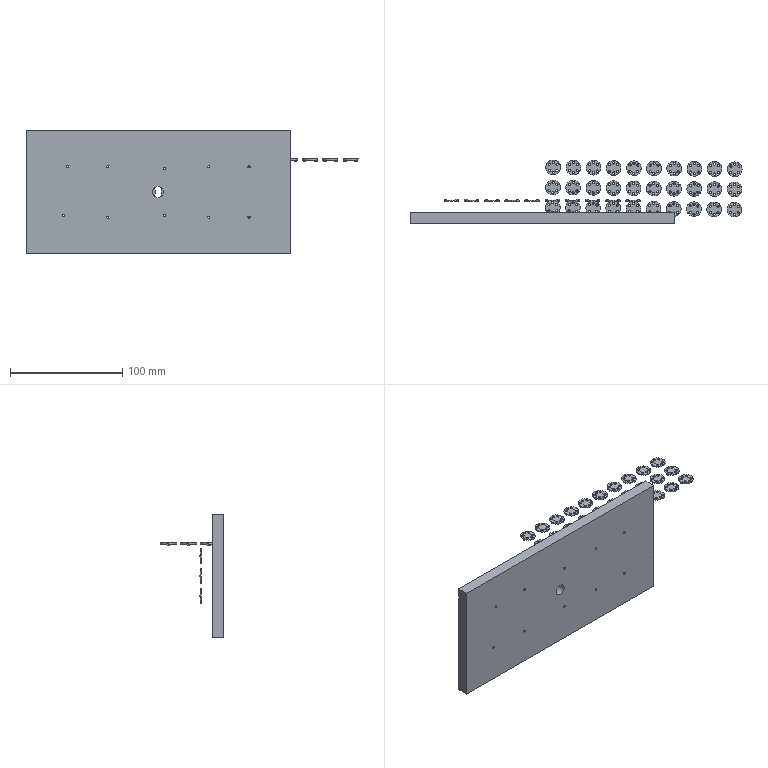NC program | NX | posted with a generic post | part box 296.27 x 56.878 x 110 mm
Lines 1 to 954 of 20851:
N10 G17 G21 G94 G90
(CAVITY_MILL_2 , TOOL : D3.R0)
N12 T03 M6
N14 G53
N16 G17 G0 G90 X-4.4 Y0. B0. C0. S4000 M3
N18 G43 Z10.1 H3
N20 G94 G1 Z-0.15 F5000.
N22 X-2.15 F2000.
N24 Y27.5
N26 G2 X-2. Y27.65 R0.15
N28 G1 X183.
N30 G2 X183.15 Y27.5 R0.15
N32 G1 Y-27.5
N34 G2 X183. Y-27.65 R0.15
N36 G1 X174.449
N38 G2 X168.332 Y-27.65 R8.4
N40 G1 X155.912
N42 G2 X150.871 Y-27.65 R8.4
N44 G1 X137.203
N46 G2 X133.582 Y-27.65 R8.4
N48 G1 X117.756
N50 G2 X117.031 Y-27.65 R8.4
N52 G1 X-2.
N54 G2 X-2.15 Y-27.5 R0.15
N56 G1 Y0.
N58 X-0.65
N60 Y26.15
N62 X8.318
N64 G3 X2.203 Y21.507 R8.4
N66 G1 X0.85 Y22.155
N68 Y24.65
N70 X2.557
N72 G3 X0.85 Y22.155 R9.9
N74 G1 X2.203 Y21.507
N76 G3 X11.239 Y26.15 R-8.4
N78 G1 X11.187 Y25.855
N80 G2 X17.755 Y16.47 R8.1
N82 X11.187 Y25.855 R-8.1
N84 G1 X11.239 Y26.15
N86 X23.077
N88 Y24.65
N90 G3 X19.558 Y19.419 R8.4
N92 X17. Y24.65 R9.9
N94 G1 X19.804
N96 Y23.3
N98 X19.71 Y23.163
N100 X19.636 Y23.3
N102 X19.804
N104 Y24.65
N106 X23.077
N108 Y26.15
N110 X181.65
N112 Y-26.15
N114 X176.92
N116 G3 X178.823 Y-23.741 R8.4
N118 G1 X180.15 Y-24.439
N120 Y-24.65
N122 X180.036
N124 G3 X180.15 Y-24.439 R9.9
N126 G1 X178.823 Y-23.741
N128 G3 X165.861 Y-26.15 R-8.4
N130 G1 X166.058 Y-25.924
N132 G2 X165.293 Y-14.495 R8.1
N134 X166.058 Y-25.924 R-8.1
N136 G1 X165.861 Y-26.15
N138 X158.696
N140 G3 X160.99 Y-23.217 R8.4
N142 G1 X162.347 Y-23.856
N144 G3 X162.745 Y-24.65 R9.9
N146 G1 X161.928
N148 G3 X162.347 Y-23.856 R9.9
N150 G1 X160.99 Y-23.217
N152 G3 X148.086 Y-26.15 R-8.4
N154 G1 X148.276 Y-25.917
N156 G2 X147.111 Y-14.522 R8.1
N158 X148.276 Y-25.917 R-8.1
N160 G1 X148.086 Y-26.15
N162 X140.455
N164 G3 X142.991 Y-23.027 R8.4
N166 G1 X144.348 Y-23.666
N168 G3 X144.854 Y-24.65 R9.9
N170 G1 X143.815
N172 G3 X144.348 Y-23.666 R9.9
N174 G1 X142.991 Y-23.027
N176 G3 X130.329 Y-26.15 R-8.4
N178 G1 X130.51 Y-25.911
N180 G2 X128.929 Y-14.565 R8.1
N182 X130.51 Y-25.911 R-8.1
N184 G1 X130.329 Y-26.15
N186 X122.195
N188 G3 X124.992 Y-22.837 R8.4
N190 G1 X126.349 Y-23.477
N192 G3 X126.881 Y-24.505 R9.9
N194 G1 X126.97 Y-24.65
N196 X125.696
N198 G3 X126.349 Y-23.477 R9.9
N200 G1 X124.992 Y-22.837
N202 G3 X112.591 Y-26.15 R-8.4
N204 G1 X112.763 Y-25.904
N206 G2 X110.747 Y-14.627 R8.1
N208 X112.763 Y-25.904 R-8.1
N210 G1 X112.591 Y-26.15
N212 X103.912
N214 G3 X106.993 Y-22.648 R8.4
N216 G1 X108.35 Y-23.287
N218 G3 X109.024 Y-24.547 R9.9
N220 G1 X109.091 Y-24.65
N222 X107.571
N224 G3 X108.35 Y-23.287 R9.9
N226 G1 X106.993 Y-22.648
N228 G3 X94.877 Y-26.15 R-8.4
N230 G1 X95.038 Y-25.897
N232 G2 X92.565 Y-14.712 R8.1
N234 X95.038 Y-25.897 R-8.1
N236 G1 X94.877 Y-26.15
N238 X85.601
N240 G3 X88.994 Y-22.458 R8.4
N242 G1 X90.351 Y-23.097
N244 G3 X91.218 Y-24.65 R9.9
N246 G1 X89.439
N248 G3 X90.351 Y-23.097 R9.9
N250 G1 X88.994 Y-22.458
N252 G3 X77.19 Y-26.15 R-8.4
N254 G1 X77.34 Y-25.89
N256 G2 X74.384 Y-14.823 R8.1
N258 X77.34 Y-25.89 R-8.1
N260 G1 X77.19 Y-26.15
N262 X67.255
N264 G3 X70.995 Y-22.269 R8.4
N266 G1 X72.352 Y-22.908
N268 G3 X73.352 Y-24.65 R9.9
N270 G1 X71.3
N272 G3 X72.352 Y-22.908 R9.9
N274 G1 X70.995 Y-22.269
N276 G3 X59.537 Y-26.15 R-8.4
N278 G1 X59.675 Y-25.884
N280 G2 X56.202 Y-14.968 R8.1
N282 X59.675 Y-25.884 R-8.1
N284 G1 X59.537 Y-26.15
N286 X48.865
N288 G3 X52.996 Y-22.079 R8.4
N290 G1 X54.353 Y-22.718
N292 G3 X55.492 Y-24.65 R9.9
N294 G1 X53.155
N296 G3 X54.353 Y-22.718 R9.9
N298 G1 X52.996 Y-22.079
N300 G3 X41.929 Y-26.15 R-8.4
N302 G1 X42.053 Y-25.877
N304 G2 X38.02 Y-15.155 R8.1
N306 X42.053 Y-25.877 R-8.1
N308 G1 X41.929 Y-26.15
N310 X30.413
N312 G3 X34.997 Y-21.889 R8.4
N314 G1 X36.354 Y-22.529
N316 G3 X37.64 Y-24.65 R9.9
N318 G1 X35.002
N320 G3 X36.354 Y-22.529 R9.9
N322 G1 X34.997 Y-21.889
N324 G3 X24.383 Y-26.15 R-8.4
N326 G1 X24.491 Y-25.87
N328 G2 X19.838 Y-15.402 R8.1
N330 X24.491 Y-25.87 R-8.1
N332 G1 X24.383 Y-26.15
N334 X11.865
N336 G3 X16.998 Y-21.7 R8.4
N338 G1 X18.355 Y-22.339
N340 G3 X19.795 Y-24.65 R9.9
N342 G1 X16.84
N344 G3 X18.355 Y-22.339 R9.9
N346 G1 X16.998 Y-21.7
N348 G3 X10.882 Y-9.852 R8.4
N350 G1 X11.146 Y-8.375
N352 G3 X11.32 Y8.099 R8.4
N354 X19.523 Y16.131 R9.9
N356 X32.478 Y24.65 R-8.4
N358 G1 X32.31 Y24.401
N360 G2 X34.491 Y13.156 R8.1
N362 X32.31 Y24.401 R-8.1
N364 G1 X32.478 Y24.65
N366 X41.37
N368 G3 X38.177 Y21.078 R8.4
N370 G1 X36.82 Y21.718
N372 G3 X36.035 Y23.15 R9.9
N374 G1 X37.648
N376 G3 X36.82 Y21.718 R9.9
N378 G1 X38.177 Y21.078
N380 G3 X50.183 Y24.65 R-8.4
N382 G1 X50.026 Y24.395
N384 G2 X52.672 Y13.249 R8.1
N386 X50.026 Y24.395 R-8.1
N388 G1 X50.183 Y24.65
N390 X59.693
N392 G3 X56.176 Y20.889 R8.4
N394 G1 X54.819 Y21.528
N396 G3 X53.905 Y23.15 R9.9
N398 G1 X55.782
N400 G3 X54.819 Y21.528 R9.9
N402 G1 X56.176 Y20.889
N404 G3 X67.858 Y24.65 R-8.4
N406 G1 X67.713 Y24.388
N408 G2 X70.854 Y13.372 R8.1
N410 X67.713 Y24.388 R-8.1
N412 G1 X67.858 Y24.65
N414 X78.053
N416 G3 X74.175 Y20.699 R8.4
N418 G1 X72.818 Y21.338
N420 G3 X71.769 Y23.15 R9.9
N422 G1 X73.923
N424 G3 X72.818 Y21.338 R9.9
N426 G1 X74.175 Y20.699
N428 G3 X85.496 Y24.65 R-8.4
N430 G1 X85.363 Y24.381
N432 G2 X89.036 Y13.531 R8.1
N434 X85.363 Y24.381 R-8.1
N436 G1 X85.496 Y24.65
N438 X96.463
N440 G3 X92.174 Y20.509 R8.4
N442 G1 X90.817 Y21.149
N444 G3 X89.626 Y23.15 R9.9
N446 G1 X92.072
N448 G3 X90.817 Y21.149 R9.9
N450 G1 X92.174 Y20.509
N452 G3 X103.084 Y24.65 R-8.4
N454 G1 X102.966 Y24.374
N456 G2 X107.218 Y13.738 R8.1
N458 X102.966 Y24.374 R-8.1
N460 G1 X103.084 Y24.65
N462 X114.945
N464 G3 X110.173 Y20.32 R8.4
N466 G1 X108.816 Y20.959
N468 G3 X107.475 Y23.15 R9.9
N470 G1 X110.228
N472 G3 X108.816 Y20.959 R9.9
N474 G1 X110.173 Y20.32
N476 G3 X120.6 Y24.65 R-8.4
N478 G1 X120.499 Y24.368
N480 G2 X125.4 Y14.014 R8.1
N482 X120.499 Y24.368 R-8.1
N484 G1 X120.6 Y24.65
N486 X133.545
N488 G3 X128.172 Y20.13 R8.4
N490 G1 X126.815 Y20.769
N492 G3 X125.317 Y23.15 R9.9
N494 G1 X128.392
N496 G3 X126.815 Y20.769 R9.9
N498 G1 X128.172 Y20.13
N500 G3 X137.998 Y24.65 R-8.4
N502 G1 X137.919 Y24.361
N504 G2 X143.582 Y14.403 R8.1
N506 X137.919 Y24.361 R-8.1
N508 G1 X137.998 Y24.65
N510 X152.41
N512 G3 X146.171 Y19.941 R8.4
N514 G1 X144.814 Y20.58
N516 G3 X143.151 Y23.15 R9.9
N518 G1 X146.565
N520 G3 X144.814 Y20.58 R9.9
N522 G1 X146.171 Y19.941
N524 G3 X155.131 Y24.65 R-8.4
N526 G1 X155.083 Y24.354
N528 G2 X161.764 Y15.049 R8.1
N530 X155.083 Y24.354 R-8.1
N532 G1 X155.131 Y24.65
N534 X180.15
N536 Y16.744
N538 G3 X164.17 Y19.751 R8.4
N540 G1 X162.813 Y20.39
N542 G3 X160.976 Y23.15 R9.9
N544 G1 X164.748
N546 G3 X162.813 Y20.39 R9.9
N548 G1 X164.17 Y19.751
N550 G3 X180.15 Y15.599 R-8.4
N552 G1 X179.851 Y15.619
N554 G2 X171.217 Y8.09 R8.1
N556 X179.851 Y15.619 R-8.1
N558 G1 X180.15 Y15.599
N560 Y-15.214
N562 G3 X173.137 Y-10.082 R9.9
N564 X177.579 Y-7.708 R8.4
N566 G1 X178.65 Y-8.758
N568 Y-11.037
N570 G3 X177.168 Y-10. R11.4
N572 X178.65 Y-8.758 R9.9
N574 G1 X177.579 Y-7.708
N576 G3 X175.16 Y5.771 R8.4
N578 G1 X175.799 Y7.128
N580 G3 X178.65 Y9.053 R9.9
N582 G1 Y5.102
N584 G3 X175.799 Y7.128 R9.9
N586 G1 X175.16 Y5.771
N588 G3 X169.849 Y-10.047 R-8.4
N590 G1 X169.911 Y-9.754
N592 G2 X163.654 Y-0.159 R8.1
N594 X169.911 Y-9.754 R-8.1
N596 G1 X169.849 Y-10.047
N598 G3 X162.434 Y-15.608 R9.9
N600 X155.138 Y-9.892 R9.9
N602 X161.18 Y-5.218 R8.4
N604 G1 X162.537 Y-5.857
N606 G3 X165.821 Y-9.88 R9.9
N608 X162.465 Y-12.735 R11.4
N610 X159.169 Y-9.81 R11.4
N612 X162.537 Y-5.857 R9.9
N614 G1 X162.507 Y-8.73
N616 G3 X163.362 Y-9.729 R11.4
N618 X162.488 Y-10.491 R12.9
N620 X161.63 Y-9.711 R12.9
N622 X162.507 Y-8.73 R11.4
N624 G1 X162.537 Y-5.857
N626 X161.18 Y-5.218
N628 G3 X157.161 Y5.961 R8.4
N630 G1 X157.8 Y7.318
N632 G3 X162.727 Y12.142 R9.9
N634 X167.551 Y7.215 R9.9
N636 X162.624 Y2.391 R9.9
N638 X157.8 Y7.318 R9.9
N640 G1 X160.672 Y7.288
N642 G3 X162.696 Y9.269 R11.4
N644 X164.678 Y7.246 R11.4
N646 X162.654 Y5.264 R11.4
N648 X160.672 Y7.288 R11.4
N650 G1 X157.8 Y7.318
N652 X157.161 Y5.961
N654 G3 X151.85 Y-9.858 R-8.4
N656 G1 X151.912 Y-9.564
N658 G2 X145.655 Y0.031 R8.1
N660 X151.912 Y-9.564 R-8.1
N662 G1 X151.85 Y-9.858
N664 G3 X144.435 Y-15.418 R9.9
N666 X137.139 Y-9.703 R9.9
N668 X143.181 Y-5.028 R8.4
N670 G1 X144.538 Y-5.667
N672 G3 X147.822 Y-9.69 R9.9
N674 X144.466 Y-12.545 R11.4
N676 X141.17 Y-9.62 R11.4
N678 X144.538 Y-5.667 R9.9
N680 G1 X144.508 Y-8.54
N682 G3 X145.363 Y-9.539 R11.4
N684 X144.489 Y-10.301 R12.9
N686 X143.631 Y-9.521 R12.9
N688 X144.508 Y-8.54 R11.4
N690 G1 X144.538 Y-5.667
N692 X143.181 Y-5.028
N694 G3 X139.162 Y6.151 R8.4
N696 G1 X139.801 Y7.508
N698 G3 X144.728 Y12.332 R9.9
N700 X149.552 Y7.405 R9.9
N702 X144.625 Y2.581 R9.9
N704 X139.801 Y7.508 R9.9
N706 G1 X142.673 Y7.477
N708 G3 X144.697 Y9.459 R11.4
N710 X146.679 Y7.435 R11.4
N712 X144.655 Y5.454 R11.4
N714 X142.673 Y7.477 R11.4
N716 G1 X139.801 Y7.508
N718 X139.162 Y6.151
N720 G3 X133.851 Y-9.668 R-8.4
N722 G1 X133.913 Y-9.375
N724 G2 X127.656 Y0.221 R8.1
N726 X133.913 Y-9.375 R-8.1
N728 G1 X133.851 Y-9.668
N730 G3 X126.436 Y-15.229 R9.9
N732 X119.14 Y-9.513 R9.9
N734 X125.182 Y-4.838 R8.4
N736 G1 X126.539 Y-5.478
N738 G3 X129.823 Y-9.501 R9.9
N740 X126.467 Y-12.356 R11.4
N742 X123.171 Y-9.431 R11.4
N744 X126.539 Y-5.478 R9.9
N746 G1 X126.509 Y-8.35
N748 G3 X127.364 Y-9.35 R11.4
N750 X126.49 Y-10.111 R12.9
N752 X125.632 Y-9.332 R12.9
N754 X126.509 Y-8.35 R11.4
N756 G1 X126.539 Y-5.478
N758 X125.182 Y-4.838
N760 G3 X121.163 Y6.34 R8.4
N762 G1 X121.802 Y7.697
N764 G3 X126.729 Y12.521 R9.9
N766 X131.553 Y7.595 R9.9
N768 X126.626 Y2.77 R9.9
N770 X121.802 Y7.697 R9.9
N772 G1 X124.674 Y7.667
N774 G3 X126.698 Y9.649 R11.4
N776 X128.68 Y7.625 R11.4
N778 X126.656 Y5.643 R11.4
N780 X124.674 Y7.667 R11.4
N782 G1 X121.802 Y7.697
N784 X121.163 Y6.34
N786 G3 X115.852 Y-9.479 R-8.4
N788 G1 X115.914 Y-9.185
N790 G2 X109.657 Y0.41 R8.1
N792 X115.914 Y-9.185 R-8.1
N794 G1 X115.852 Y-9.479
N796 G3 X108.437 Y-15.039 R9.9
N798 X101.141 Y-9.324 R9.9
N800 X107.183 Y-4.649 R8.4
N802 G1 X108.54 Y-5.288
N804 G3 X111.823 Y-9.311 R9.9
N806 X108.468 Y-12.166 R11.4
N808 X105.172 Y-9.241 R11.4
N810 X108.54 Y-5.288 R9.9
N812 G1 X108.51 Y-8.161
N814 G3 X109.365 Y-9.16 R11.4
N816 X108.491 Y-9.922 R12.9
N818 X107.633 Y-9.142 R12.9
N820 X108.51 Y-8.161 R11.4
N822 G1 X108.54 Y-5.288
N824 X107.183 Y-4.649
N826 G3 X103.164 Y6.53 R8.4
N828 G1 X103.803 Y7.887
N830 G3 X108.73 Y12.711 R9.9
N832 X113.554 Y7.784 R9.9
N834 X108.627 Y2.96 R9.9
N836 X103.803 Y7.887 R9.9
N838 G1 X106.675 Y7.857
N840 G3 X108.699 Y9.838 R11.4
N842 X110.681 Y7.814 R11.4
N844 X108.657 Y5.833 R11.4
N846 X106.675 Y7.857 R11.4
N848 G1 X103.803 Y7.887
N850 X103.164 Y6.53
N852 G3 X97.853 Y-9.289 R-8.4
N854 G1 X97.915 Y-8.995
N856 G2 X91.658 Y0.6 R8.1
N858 X97.915 Y-8.995 R-8.1
N860 G1 X97.853 Y-9.289
N862 G3 X90.438 Y-14.849 R9.9
N864 X83.142 Y-9.134 R9.9
N866 X89.184 Y-4.459 R8.4
N868 G1 X90.541 Y-5.098
N870 G3 X93.824 Y-9.121 R9.9
N872 X90.469 Y-11.977 R11.4
N874 X87.173 Y-9.051 R11.4
N876 X90.541 Y-5.098 R9.9
N878 G1 X90.511 Y-7.971
N880 G3 X91.366 Y-8.971 R11.4
N882 X90.492 Y-9.732 R12.9
N884 X89.634 Y-8.952 R12.9
N886 X90.511 Y-7.971 R11.4
N888 G1 X90.541 Y-5.098
N890 X89.184 Y-4.459
N892 G3 X85.165 Y6.72 R8.4
N894 G1 X85.804 Y8.076
N896 G3 X90.731 Y12.901 R9.9
N898 X95.555 Y7.974 R9.9
N900 X90.628 Y3.15 R9.9
N902 X85.804 Y8.076 R9.9
N904 G1 X88.676 Y8.046
N906 G3 X90.7 Y10.028 R11.4
N908 X92.682 Y8.004 R11.4
N910 X90.658 Y6.022 R11.4
N912 X88.676 Y8.046 R11.4
N914 G1 X85.804 Y8.076
N916 X85.165 Y6.72
N918 G3 X79.854 Y-9.099 R-8.4
N920 G1 X79.916 Y-8.806
N922 G2 X73.659 Y0.79 R8.1
N924 X79.916 Y-8.806 R-8.1
N926 G1 X79.854 Y-9.099
N928 G3 X72.439 Y-14.66 R9.9
N930 X65.143 Y-8.944 R9.9
N932 X71.185 Y-4.27 R8.4
N934 G1 X72.542 Y-4.909
N936 G3 X75.825 Y-8.932 R9.9
N938 X72.47 Y-11.787 R11.4
N940 X69.174 Y-8.862 R11.4
N942 X72.542 Y-4.909 R9.9
N944 G1 X72.512 Y-7.782
N946 G3 X73.367 Y-8.781 R11.4
N948 X72.493 Y-9.543 R12.9
N950 X71.635 Y-8.763 R12.9
N952 X72.512 Y-7.782 R11.4
N954 G1 X72.542 Y-4.909
N956 X71.185 Y-4.27
N958 G3 X67.166 Y6.909 R8.4
N960 G1 X67.805 Y8.266
N962 G3 X72.732 Y13.09 R9.9
N964 X77.556 Y8.163 R9.9
N966 X72.629 Y3.339 R9.9
N968 X67.805 Y8.266 R9.9
N970 G1 X70.677 Y8.236
N972 G3 X72.701 Y10.217 R11.4
N974 X74.683 Y8.194 R11.4
N976 X72.659 Y6.212 R11.4
N978 X70.677 Y8.236 R11.4
N980 G1 X67.805 Y8.266
N982 X67.166 Y6.909
N984 G3 X61.855 Y-8.91 R-8.4
N986 G1 X61.917 Y-8.616
N988 G2 X55.66 Y0.979 R8.1
N990 X61.917 Y-8.616 R-8.1
N992 G1 X61.855 Y-8.91
N994 G3 X54.44 Y-14.47 R9.9
N996 X47.237 Y-8.772 R9.9
N998 G1 X47.144 Y-8.755
N1000 G3 X53.186 Y-4.08 R8.4
N1002 G1 X54.543 Y-4.719
N1004 G3 X57.826 Y-8.742 R9.9
N1006 X54.471 Y-11.597 R11.4
N1008 X51.175 Y-8.672 R11.4
N1010 X54.543 Y-4.719 R9.9
N1012 G1 X54.513 Y-7.592
N1014 G3 X55.368 Y-8.591 R11.4
N1016 X54.494 Y-9.353 R12.9
N1018 X53.636 Y-8.573 R12.9
N1020 X54.513 Y-7.592 R11.4
N1022 G1 X54.543 Y-4.719
N1024 X53.186 Y-4.08
N1026 G3 X49.167 Y7.099 R8.4
N1028 G1 X49.806 Y8.456
N1030 G3 X54.733 Y13.28 R9.9
N1032 X59.557 Y8.353 R9.9
N1034 X54.63 Y3.529 R9.9
N1036 X49.806 Y8.456 R9.9
N1038 G1 X52.678 Y8.425
N1040 G3 X54.702 Y10.407 R11.4
N1042 X56.684 Y8.383 R11.4
N1044 X54.66 Y6.402 R11.4
N1046 X52.678 Y8.425 R11.4
N1048 G1 X49.806 Y8.456
N1050 X49.167 Y7.099
N1052 G3 X43.856 Y-8.72 R-8.4
N1054 G1 X43.918 Y-8.426
N1056 G2 X37.661 Y1.169 R8.1
N1058 X43.918 Y-8.426 R-8.1
N1060 G1 X43.856 Y-8.72
N1062 G3 X36.441 Y-14.28 R9.9
N1064 X29.145 Y-8.565 R9.9
N1066 X35.187 Y-3.89 R8.4
N1068 G1 X36.544 Y-4.53
N1070 G3 X39.827 Y-8.553 R9.9
N1072 X36.472 Y-11.408 R11.4
N1074 X33.176 Y-8.483 R11.4
N1076 X36.544 Y-4.53 R9.9
N1078 G1 X36.514 Y-7.402
N1080 G3 X37.369 Y-8.402 R11.4
N1082 X36.495 Y-9.163 R12.9
N1084 X35.637 Y-8.383 R12.9
N1086 X36.514 Y-7.402 R11.4
N1088 G1 X36.544 Y-4.53
N1090 X35.187 Y-3.89
N1092 G3 X31.168 Y7.288 R8.4
N1094 G1 X31.807 Y8.645
N1096 G3 X36.734 Y13.469 R9.9
N1098 X41.558 Y8.543 R9.9
N1100 X36.631 Y3.719 R9.9
N1102 X31.807 Y8.645 R9.9
N1104 G1 X34.679 Y8.615
N1106 G3 X36.703 Y10.597 R11.4
N1108 X38.685 Y8.573 R11.4
N1110 X36.661 Y6.591 R11.4
N1112 X34.679 Y8.615 R11.4
N1114 G1 X31.807 Y8.645
N1116 X31.168 Y7.288
N1118 G3 X19.989 Y3.269 R8.4
N1120 G1 X18.632 Y3.908
N1122 G3 X15.348 Y7.931 R9.9
N1124 X19.606 Y12.1 R11.4
N1126 X23.559 Y8.732 R9.9
N1128 X18.632 Y3.908 R9.9
N1130 G1 X18.662 Y6.781
N1132 G3 X17.806 Y7.78 R11.4
N1134 X19.705 Y9.639 R12.9
N1136 X20.686 Y8.763 R11.4
N1138 X18.662 Y6.781 R11.4
N1140 G1 X18.632 Y3.908
N1142 X19.989 Y3.269
N1144 G3 X25.857 Y-8.53 R8.4
N1146 G1 X25.919 Y-8.237
N1148 G2 X19.662 Y1.358 R8.1
N1150 X25.919 Y-8.237 R-8.1
N1152 G1 X25.857 Y-8.53
N1154 G3 X18.442 Y-14.091 R9.9
N1156 X14.417 Y-9.586 R9.9
N1158 G1 X15.177 Y-8.293
N1160 G3 X18.545 Y-4.34 R9.9
N1162 X21.828 Y-8.363 R9.9
N1164 X18.472 Y-11.218 R11.4
N1166 X15.177 Y-8.293 R11.4
N1168 G1 X17.638 Y-8.194
N1170 G3 X18.515 Y-7.213 R11.4
N1172 X19.37 Y-8.212 R11.4
N1174 X18.496 Y-8.974 R12.9
N1176 X17.638 Y-8.194 R12.9
N1178 G1 X15.177 Y-8.293
N1180 X14.417 Y-9.586
N1182 G3 X11.146 Y-8.375 R9.9
N1184 G1 X10.882 Y-9.852
N1186 G3 X6.933 Y-26.15 R8.4
N1188 G1 X7.022 Y-25.863
N1190 G2 X1.656 Y-15.742 R8.1
N1192 X7.022 Y-25.863 R-8.1
N1194 G1 X6.933 Y-26.15
N1196 X-0.65
N1198 Y-23.112
N1200 X0.85
N1202 G3 X1.958 Y-24.65 R9.9
N1204 G1 X0.85
N1206 Y-23.112
N1208 X-0.65
N1210 Y0.
N1212 X0.85
N1214 Y13.601
N1216 G3 X8.032 Y8.133 R9.9
N1218 X3.447 Y5.609 R8.4
N1220 G1 X2.35 Y6.632
N1222 Y9.231
N1224 G3 X4. Y8.051 R11.4
N1226 X2.35 Y6.632 R9.9
N1228 G1 X3.447 Y5.609
N1230 G3 X7.858 Y-8.341 R8.4
N1232 G1 X7.92 Y-8.047
N1234 G2 X1.663 Y1.548 R8.1
N1236 X7.92 Y-8.047 R-8.1
N1238 G1 X7.858 Y-8.341
N1240 G3 X0.85 Y-13.128 R9.9
N1242 G1 Y-6.874
N1244 X2.35
N1246 G3 X3.829 Y-8.173 R9.9
N1248 X2.35 Y-9.161 R11.4
N1250 G1 Y-6.874
N1252 X0.85
N1254 Y0.
N1256 X-1.4
N1258 G0 Z0.1
N1260 X-4.4
N1262 G1 Z-0.3 F5000.
N1264 X-2.15 F2000.
N1266 Y27.5
N1268 G2 X-2. Y27.65 R0.15
N1270 G1 X183.
N1272 G2 X183.15 Y27.5 R0.15
N1274 G1 Y-27.5
N1276 G2 X183. Y-27.65 R0.15
N1278 G1 X174.449
N1280 G2 X168.332 Y-27.65 R8.4
N1282 G1 X155.912
N1284 G2 X150.871 Y-27.65 R8.4
N1286 G1 X137.203
N1288 G2 X133.582 Y-27.65 R8.4
N1290 G1 X117.756
N1292 G2 X117.031 Y-27.65 R8.4
N1294 G1 X-2.
N1296 G2 X-2.15 Y-27.5 R0.15
N1298 G1 Y0.
N1300 X-0.65
N1302 Y26.15
N1304 X8.318
N1306 G3 X2.203 Y21.507 R8.4
N1308 G1 X0.85 Y22.155
N1310 Y24.65
N1312 X2.557
N1314 G3 X0.85 Y22.155 R9.9
N1316 G1 X2.203 Y21.507
N1318 G3 X11.239 Y26.15 R-8.4
N1320 G1 X11.187 Y25.855
N1322 G2 X17.755 Y16.47 R8.1
N1324 X11.187 Y25.855 R-8.1
N1326 G1 X11.239 Y26.15
N1328 X23.077
N1330 Y24.65
N1332 G3 X19.558 Y19.419 R8.4
N1334 X17. Y24.65 R9.9
N1336 G1 X19.804
N1338 Y23.3
N1340 X19.71 Y23.163
N1342 X19.636 Y23.3
N1344 X19.804
N1346 Y24.65
N1348 X23.077
N1350 Y26.15
N1352 X181.65
N1354 Y-26.15
N1356 X176.92
N1358 G3 X178.823 Y-23.741 R8.4
N1360 G1 X180.15 Y-24.439
N1362 Y-24.65
N1364 X180.036
N1366 G3 X180.15 Y-24.439 R9.9
N1368 G1 X178.823 Y-23.741
N1370 G3 X165.861 Y-26.15 R-8.4
N1372 G1 X166.058 Y-25.924
N1374 G2 X165.293 Y-14.495 R8.1
N1376 X166.058 Y-25.924 R-8.1
N1378 G1 X165.861 Y-26.15
N1380 X158.696
N1382 G3 X160.99 Y-23.217 R8.4
N1384 G1 X162.347 Y-23.856
N1386 G3 X162.745 Y-24.65 R9.9
N1388 G1 X161.928
N1390 G3 X162.347 Y-23.856 R9.9
N1392 G1 X160.99 Y-23.217
N1394 G3 X148.086 Y-26.15 R-8.4
N1396 G1 X148.276 Y-25.917
N1398 G2 X147.111 Y-14.522 R8.1
N1400 X148.276 Y-25.917 R-8.1
N1402 G1 X148.086 Y-26.15
N1404 X140.455
N1406 G3 X142.991 Y-23.027 R8.4
N1408 G1 X144.348 Y-23.666
N1410 G3 X144.854 Y-24.65 R9.9
N1412 G1 X143.815
N1414 G3 X144.348 Y-23.666 R9.9
N1416 G1 X142.991 Y-23.027
N1418 G3 X130.329 Y-26.15 R-8.4
N1420 G1 X130.51 Y-25.911
N1422 G2 X128.929 Y-14.565 R8.1
N1424 X130.51 Y-25.911 R-8.1
N1426 G1 X130.329 Y-26.15
N1428 X122.195
N1430 G3 X124.992 Y-22.837 R8.4
N1432 G1 X126.349 Y-23.477
N1434 G3 X126.881 Y-24.505 R9.9
N1436 G1 X126.97 Y-24.65
N1438 X125.696
N1440 G3 X126.349 Y-23.477 R9.9
N1442 G1 X124.992 Y-22.837
N1444 G3 X112.591 Y-26.15 R-8.4
N1446 G1 X112.763 Y-25.904
N1448 G2 X110.747 Y-14.627 R8.1
N1450 X112.763 Y-25.904 R-8.1
N1452 G1 X112.591 Y-26.15
N1454 X103.912
N1456 G3 X106.993 Y-22.648 R8.4
N1458 G1 X108.35 Y-23.287
N1460 G3 X109.024 Y-24.547 R9.9
N1462 G1 X109.091 Y-24.65
N1464 X107.571
N1466 G3 X108.35 Y-23.287 R9.9
N1468 G1 X106.993 Y-22.648
N1470 G3 X94.877 Y-26.15 R-8.4
N1472 G1 X95.038 Y-25.897
N1474 G2 X92.565 Y-14.712 R8.1
N1476 X95.038 Y-25.897 R-8.1
N1478 G1 X94.877 Y-26.15
N1480 X85.601
N1482 G3 X88.994 Y-22.458 R8.4
N1484 G1 X90.351 Y-23.097
N1486 G3 X91.218 Y-24.65 R9.9
N1488 G1 X89.439
N1490 G3 X90.351 Y-23.097 R9.9
N1492 G1 X88.994 Y-22.458
N1494 G3 X77.19 Y-26.15 R-8.4
N1496 G1 X77.34 Y-25.89
N1498 G2 X74.384 Y-14.823 R8.1
N1500 X77.34 Y-25.89 R-8.1
N1502 G1 X77.19 Y-26.15
N1504 X67.255
N1506 G3 X70.995 Y-22.269 R8.4
N1508 G1 X72.352 Y-22.908
N1510 G3 X73.352 Y-24.65 R9.9
N1512 G1 X71.3
N1514 G3 X72.352 Y-22.908 R9.9
N1516 G1 X70.995 Y-22.269
N1518 G3 X59.537 Y-26.15 R-8.4
N1520 G1 X59.675 Y-25.884
N1522 G2 X56.202 Y-14.968 R8.1
N1524 X59.675 Y-25.884 R-8.1
N1526 G1 X59.537 Y-26.15
N1528 X48.865
N1530 G3 X52.996 Y-22.079 R8.4
N1532 G1 X54.353 Y-22.718
N1534 G3 X55.492 Y-24.65 R9.9
N1536 G1 X53.155
N1538 G3 X54.353 Y-22.718 R9.9
N1540 G1 X52.996 Y-22.079
N1542 G3 X41.929 Y-26.15 R-8.4
N1544 G1 X42.053 Y-25.877
N1546 G2 X38.02 Y-15.155 R8.1
N1548 X42.053 Y-25.877 R-8.1
N1550 G1 X41.929 Y-26.15
N1552 X30.413
N1554 G3 X34.997 Y-21.889 R8.4
N1556 G1 X36.354 Y-22.529
N1558 G3 X37.64 Y-24.65 R9.9
N1560 G1 X35.002
N1562 G3 X36.354 Y-22.529 R9.9
N1564 G1 X34.997 Y-21.889
N1566 G3 X24.383 Y-26.15 R-8.4
N1568 G1 X24.491 Y-25.87
N1570 G2 X19.838 Y-15.402 R8.1
N1572 X24.491 Y-25.87 R-8.1
N1574 G1 X24.383 Y-26.15
N1576 X11.865
N1578 G3 X16.998 Y-21.7 R8.4
N1580 G1 X18.355 Y-22.339
N1582 G3 X19.795 Y-24.65 R9.9
N1584 G1 X16.84
N1586 G3 X18.355 Y-22.339 R9.9
N1588 G1 X16.998 Y-21.7
N1590 G3 X10.882 Y-9.852 R8.4
N1592 G1 X11.146 Y-8.375
N1594 G3 X11.32 Y8.099 R8.4
N1596 X19.523 Y16.131 R9.9
N1598 X32.478 Y24.65 R-8.4
N1600 G1 X32.31 Y24.401
N1602 G2 X34.491 Y13.156 R8.1
N1604 X32.31 Y24.401 R-8.1
N1606 G1 X32.478 Y24.65
N1608 X41.37
N1610 G3 X38.177 Y21.078 R8.4
N1612 G1 X36.82 Y21.718
N1614 G3 X36.035 Y23.15 R9.9
N1616 G1 X37.648
N1618 G3 X36.82 Y21.718 R9.9
N1620 G1 X38.177 Y21.078
N1622 G3 X50.183 Y24.65 R-8.4
N1624 G1 X50.026 Y24.395
N1626 G2 X52.672 Y13.249 R8.1
N1628 X50.026 Y24.395 R-8.1
N1630 G1 X50.183 Y24.65
N1632 X59.693
N1634 G3 X56.176 Y20.889 R8.4
N1636 G1 X54.819 Y21.528
N1638 G3 X53.905 Y23.15 R9.9
N1640 G1 X55.782
N1642 G3 X54.819 Y21.528 R9.9
N1644 G1 X56.176 Y20.889
N1646 G3 X67.858 Y24.65 R-8.4
N1648 G1 X67.713 Y24.388
N1650 G2 X70.854 Y13.372 R8.1
N1652 X67.713 Y24.388 R-8.1
N1654 G1 X67.858 Y24.65
N1656 X78.053
N1658 G3 X74.175 Y20.699 R8.4
N1660 G1 X72.818 Y21.338
N1662 G3 X71.769 Y23.15 R9.9
N1664 G1 X73.923
N1666 G3 X72.818 Y21.338 R9.9
N1668 G1 X74.175 Y20.699
N1670 G3 X85.496 Y24.65 R-8.4
N1672 G1 X85.363 Y24.381
N1674 G2 X89.036 Y13.531 R8.1
N1676 X85.363 Y24.381 R-8.1
N1678 G1 X85.496 Y24.65
N1680 X96.463
N1682 G3 X92.174 Y20.509 R8.4
N1684 G1 X90.817 Y21.149
N1686 G3 X89.626 Y23.15 R9.9
N1688 G1 X92.072
N1690 G3 X90.817 Y21.149 R9.9
N1692 G1 X92.174 Y20.509
N1694 G3 X103.084 Y24.65 R-8.4
N1696 G1 X102.966 Y24.374
N1698 G2 X107.218 Y13.738 R8.1
N1700 X102.966 Y24.374 R-8.1
N1702 G1 X103.084 Y24.65
N1704 X114.945
N1706 G3 X110.173 Y20.32 R8.4
N1708 G1 X108.816 Y20.959
N1710 G3 X107.475 Y23.15 R9.9
N1712 G1 X110.228
N1714 G3 X108.816 Y20.959 R9.9
N1716 G1 X110.173 Y20.32
N1718 G3 X120.6 Y24.65 R-8.4
N1720 G1 X120.499 Y24.368
N1722 G2 X125.4 Y14.014 R8.1
N1724 X120.499 Y24.368 R-8.1
N1726 G1 X120.6 Y24.65
N1728 X133.545
N1730 G3 X128.172 Y20.13 R8.4
N1732 G1 X126.815 Y20.769
N1734 G3 X125.317 Y23.15 R9.9
N1736 G1 X128.392
N1738 G3 X126.815 Y20.769 R9.9
N1740 G1 X128.172 Y20.13
N1742 G3 X137.998 Y24.65 R-8.4
N1744 G1 X137.919 Y24.361
N1746 G2 X143.582 Y14.403 R8.1
N1748 X137.919 Y24.361 R-8.1
N1750 G1 X137.998 Y24.65
N1752 X152.41
N1754 G3 X146.171 Y19.941 R8.4
N1756 G1 X144.814 Y20.58
N1758 G3 X143.151 Y23.15 R9.9
N1760 G1 X146.565
N1762 G3 X144.814 Y20.58 R9.9
N1764 G1 X146.171 Y19.941
N1766 G3 X155.131 Y24.65 R-8.4
N1768 G1 X155.083 Y24.354
N1770 G2 X161.764 Y15.049 R8.1
N1772 X155.083 Y24.354 R-8.1
N1774 G1 X155.131 Y24.65
N1776 X180.15
N1778 Y16.744
N1780 G3 X164.17 Y19.751 R8.4
N1782 G1 X162.813 Y20.39
N1784 G3 X160.976 Y23.15 R9.9
N1786 G1 X164.748
N1788 G3 X162.813 Y20.39 R9.9
N1790 G1 X164.17 Y19.751
N1792 G3 X180.15 Y15.599 R-8.4
N1794 G1 X179.851 Y15.619
N1796 G2 X171.217 Y8.09 R8.1
N1798 X179.851 Y15.619 R-8.1
N1800 G1 X180.15 Y15.599
N1802 Y-15.214
N1804 G3 X173.137 Y-10.082 R9.9
N1806 X177.579 Y-7.708 R8.4
N1808 G1 X178.65 Y-8.758
N1810 Y-11.037
N1812 G3 X177.168 Y-10. R11.4
N1814 X178.65 Y-8.758 R9.9
N1816 G1 X177.579 Y-7.708
N1818 G3 X175.16 Y5.771 R8.4
N1820 G1 X175.799 Y7.128
N1822 G3 X178.65 Y9.053 R9.9
N1824 G1 Y5.102
N1826 G3 X175.799 Y7.128 R9.9
N1828 G1 X175.16 Y5.771
N1830 G3 X169.849 Y-10.047 R-8.4
N1832 G1 X169.911 Y-9.754
N1834 G2 X163.654 Y-0.159 R8.1
N1836 X169.911 Y-9.754 R-8.1
N1838 G1 X169.849 Y-10.047
N1840 G3 X162.434 Y-15.608 R9.9
N1842 X155.138 Y-9.892 R9.9
N1844 X161.18 Y-5.218 R8.4
N1846 G1 X162.537 Y-5.857
N1848 G3 X165.821 Y-9.88 R9.9
N1850 X162.465 Y-12.735 R11.4
N1852 X159.169 Y-9.81 R11.4
N1854 X162.537 Y-5.857 R9.9
N1856 G1 X162.507 Y-8.73
N1858 G3 X163.362 Y-9.729 R11.4
N1860 X162.488 Y-10.491 R12.9
N1862 X161.63 Y-9.711 R12.9
N1864 X162.507 Y-8.73 R11.4
N1866 G1 X162.537 Y-5.857
N1868 X161.18 Y-5.218
N1870 G3 X157.161 Y5.961 R8.4
N1872 G1 X157.8 Y7.318
N1874 G3 X162.727 Y12.142 R9.9
N1876 X167.551 Y7.215 R9.9
N1878 X162.624 Y2.391 R9.9
N1880 X157.8 Y7.318 R9.9
N1882 G1 X160.672 Y7.288
N1884 G3 X162.696 Y9.269 R11.4
N1886 X164.678 Y7.246 R11.4
N1888 X162.654 Y5.264 R11.4
N1890 X160.672 Y7.288 R11.4
N1892 G1 X157.8 Y7.318
N1894 X157.161 Y5.961
N1896 G3 X151.85 Y-9.858 R-8.4
N1898 G1 X151.912 Y-9.564
N1900 G2 X145.655 Y0.031 R8.1
N1902 X151.912 Y-9.564 R-8.1
N1904 G1 X151.85 Y-9.858
N1906 G3 X144.435 Y-15.418 R9.9